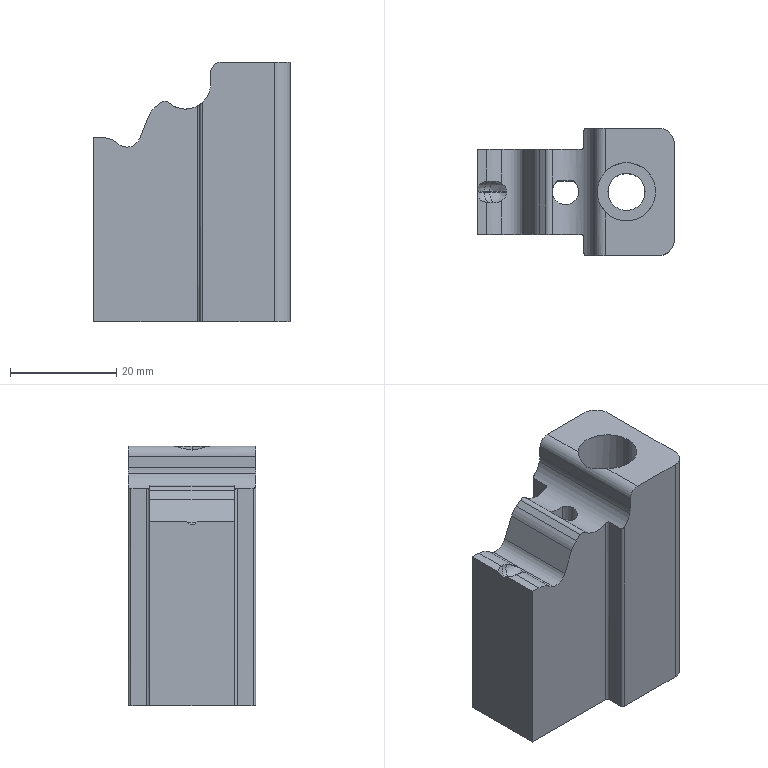Part | 1 solid | 48 faces | box 37.007 x 24 x 48.948 mm | volume 27878 mm3 | cylinder 21 | plane 19 | spline 8 | commonest cylinder face diameters 1 x4 6 x2 7 x2 8.206 x2 9 x2 9.5 x2